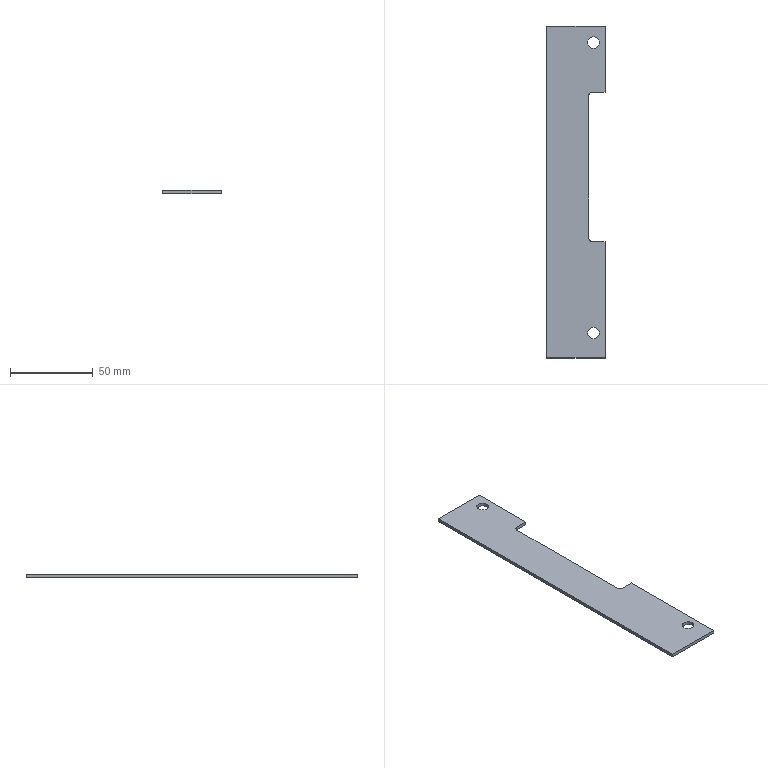Part | STEP file | 1_id642_x_t | 1 solid | 16 faces | box 35 x 200 x 2 mm | volume 12091 mm3 | plane 10 | cylinder 6 | commonest cylinder face diameters 7 x4 4 x2
STEP:
#1=CARTESIAN_POINT('',(0.,0.,0.));
#2=DIRECTION('',(0.,0.,1.));
#3=DIRECTION('',(1.,0.,0.));
#4=AXIS2_PLACEMENT_3D('',#1,#2,#3);
#5=CARTESIAN_POINT('',(533.775,132.525,-88.));
#6=VERTEX_POINT('',#5);
#7=CARTESIAN_POINT('',(531.775,134.525,-88.));
#8=VERTEX_POINT('',#7);
#9=CARTESIAN_POINT('',(533.775,134.525,-88.));
#10=DIRECTION('',(0.,0.,-1.));
#11=DIRECTION('',(0.,-1.,0.));
#12=AXIS2_PLACEMENT_3D('',#9,#10,#11);
#13=CIRCLE('',#12,2.);
#14=CARTESIAN_POINT('',(541.55,307.352,-88.));
#15=DIRECTION('',(0.,0.,1.));
#16=DIRECTION('',(1.,0.,0.));
#17=AXIS2_PLACEMENT_3D('',#14,#15,#16);
#18=PLANE('',#17);
#19=CARTESIAN_POINT('',(-7.775,-174.827));
#20=CARTESIAN_POINT('',(-11.239,-174.827));
#21=CARTESIAN_POINT('',(-9.507,-171.827));
#22=CARTESIAN_POINT('',(-7.775,-168.827));
#23=CARTESIAN_POINT('',(-6.043,-171.827));
#24=CARTESIAN_POINT('',(-4.311,-174.827));
#25=CARTESIAN_POINT('',(-7.775,-174.827));
#26=(BOUNDED_CURVE()B_SPLINE_CURVE(2,(#19,#20,#21,#22,#23,#24,#25),.UNSPECIFIED.,.T.,.F.)B_SPLINE_CURVE_WITH_KNOTS((1,2,2,2,2,1),(-2.094,0.,2.094,4.189,6.283,8.378),.UNSPECIFIED.)CURVE()GEOMETRIC_REPRESENTATION_ITEM()RATIONAL_B_SPLINE_CURVE((1.,0.5,1.,0.5,1.,0.5,1.))REPRESENTATION_ITEM(''));
#27=(GEOMETRIC_REPRESENTATION_CONTEXT(2)PARAMETRIC_REPRESENTATION_CONTEXT()REPRESENTATION_CONTEXT('',''));
#28=DEFINITIONAL_REPRESENTATION('',(#26),#27);
#29=PCURVE('',#18,#28);
#30=CARTESIAN_POINT('',(533.775,134.525,-92.));
#31=DIRECTION('',(0.,0.,-1.));
#32=DIRECTION('',(1.,0.,0.));
#33=AXIS2_PLACEMENT_3D('',#30,#31,#32);
#34=CYLINDRICAL_SURFACE('',#33,2.);
#35=CARTESIAN_POINT('',(1.571,-4.));
#36=DIRECTION('',(1.,0.));
#37=VECTOR('',#36,1.);
#38=LINE('',#35,#37);
#39=(GEOMETRIC_REPRESENTATION_CONTEXT(2)PARAMETRIC_REPRESENTATION_CONTEXT()REPRESENTATION_CONTEXT('',''));
#40=DEFINITIONAL_REPRESENTATION('',(#38),#39);
#41=PCURVE('',#34,#40);
#42=SURFACE_CURVE('',#13,(#29,#41),.PCURVE_S1.);
#43=EDGE_CURVE('',#6,#8,#42,.T.);
#44=ORIENTED_EDGE('',*,*,#43,.T.);
#45=CARTESIAN_POINT('',(531.775,220.475,-88.));
#46=VERTEX_POINT('',#45);
#47=CARTESIAN_POINT('',(531.775,134.525,-88.));
#48=DIRECTION('',(0.,1.,0.));
#49=VECTOR('',#48,1.);
#50=LINE('',#47,#49);
#51=CARTESIAN_POINT('',(-9.775,-172.827));
#52=DIRECTION('',(0.,1.));
#53=VECTOR('',#52,1.);
#54=LINE('',#51,#53);
#55=(GEOMETRIC_REPRESENTATION_CONTEXT(2)PARAMETRIC_REPRESENTATION_CONTEXT()REPRESENTATION_CONTEXT('',''));
#56=DEFINITIONAL_REPRESENTATION('',(#54),#55);
#57=PCURVE('',#18,#56);
#58=CARTESIAN_POINT('',(531.775,177.5,-92.));
#59=DIRECTION('',(-1.,0.,0.));
#60=DIRECTION('',(0.,0.,-1.));
#61=AXIS2_PLACEMENT_3D('',#58,#59,#60);
#62=PLANE('',#61);
#63=CARTESIAN_POINT('',(-4.,42.975));
#64=DIRECTION('',(0.,-1.));
#65=VECTOR('',#64,1.);
#66=LINE('',#63,#65);
#67=(GEOMETRIC_REPRESENTATION_CONTEXT(2)PARAMETRIC_REPRESENTATION_CONTEXT()REPRESENTATION_CONTEXT('',''));
#68=DEFINITIONAL_REPRESENTATION('',(#66),#67);
#69=PCURVE('',#62,#68);
#70=SURFACE_CURVE('',#50,(#57,#69),.PCURVE_S1.);
#71=EDGE_CURVE('',#8,#46,#70,.T.);
#72=ORIENTED_EDGE('',*,*,#71,.T.);
#73=CARTESIAN_POINT('',(533.775,222.475,-88.));
#74=VERTEX_POINT('',#73);
#75=CARTESIAN_POINT('',(533.775,220.475,-88.));
#76=DIRECTION('',(0.,0.,-1.));
#77=DIRECTION('',(-1.,0.,0.));
#78=AXIS2_PLACEMENT_3D('',#75,#76,#77);
#79=CIRCLE('',#78,2.);
#80=CARTESIAN_POINT('',(-9.775,-86.877));
#81=CARTESIAN_POINT('',(-9.775,-83.413));
#82=CARTESIAN_POINT('',(-6.775,-85.145));
#83=CARTESIAN_POINT('',(-3.775,-86.877));
#84=CARTESIAN_POINT('',(-6.775,-88.609));
#85=CARTESIAN_POINT('',(-9.775,-90.341));
#86=CARTESIAN_POINT('',(-9.775,-86.877));
#87=(BOUNDED_CURVE()B_SPLINE_CURVE(2,(#80,#81,#82,#83,#84,#85,#86),.UNSPECIFIED.,.T.,.F.)B_SPLINE_CURVE_WITH_KNOTS((1,2,2,2,2,1),(-2.094,0.,2.094,4.189,6.283,8.378),.UNSPECIFIED.)CURVE()GEOMETRIC_REPRESENTATION_ITEM()RATIONAL_B_SPLINE_CURVE((1.,0.5,1.,0.5,1.,0.5,1.))REPRESENTATION_ITEM(''));
#88=(GEOMETRIC_REPRESENTATION_CONTEXT(2)PARAMETRIC_REPRESENTATION_CONTEXT()REPRESENTATION_CONTEXT('',''));
#89=DEFINITIONAL_REPRESENTATION('',(#87),#88);
#90=PCURVE('',#18,#89);
#91=CARTESIAN_POINT('',(533.775,220.475,-92.));
#92=DIRECTION('',(0.,0.,-1.));
#93=DIRECTION('',(1.,0.,0.));
#94=AXIS2_PLACEMENT_3D('',#91,#92,#93);
#95=CYLINDRICAL_SURFACE('',#94,2.);
#96=CARTESIAN_POINT('',(3.142,-4.));
#97=DIRECTION('',(1.,0.));
#98=VECTOR('',#97,1.);
#99=LINE('',#96,#98);
#100=(GEOMETRIC_REPRESENTATION_CONTEXT(2)PARAMETRIC_REPRESENTATION_CONTEXT()REPRESENTATION_CONTEXT('',''));
#101=DEFINITIONAL_REPRESENTATION('',(#99),#100);
#102=PCURVE('',#95,#101);
#103=SURFACE_CURVE('',#79,(#90,#102),.PCURVE_S1.);
#104=EDGE_CURVE('',#46,#74,#103,.T.);
#105=ORIENTED_EDGE('',*,*,#104,.T.);
#106=CARTESIAN_POINT('',(541.55,222.475,-88.));
#107=VERTEX_POINT('',#106);
#108=CARTESIAN_POINT('',(533.775,222.475,-88.));
#109=DIRECTION('',(1.,0.,0.));
#110=VECTOR('',#109,1.);
#111=LINE('',#108,#110);
#112=CARTESIAN_POINT('',(-7.775,-84.877));
#113=DIRECTION('',(1.,0.));
#114=VECTOR('',#113,1.);
#115=LINE('',#112,#114);
#116=(GEOMETRIC_REPRESENTATION_CONTEXT(2)PARAMETRIC_REPRESENTATION_CONTEXT()REPRESENTATION_CONTEXT('',''));
#117=DEFINITIONAL_REPRESENTATION('',(#115),#116);
#118=PCURVE('',#18,#117);
#119=CARTESIAN_POINT('',(537.663,222.475,-92.));
#120=DIRECTION('',(0.,1.,0.));
#121=DIRECTION('',(0.,0.,-1.));
#122=AXIS2_PLACEMENT_3D('',#119,#120,#121);
#123=PLANE('',#122);
#124=CARTESIAN_POINT('',(-4.,3.888));
#125=DIRECTION('',(0.,-1.));
#126=VECTOR('',#125,1.);
#127=LINE('',#124,#126);
#128=(GEOMETRIC_REPRESENTATION_CONTEXT(2)PARAMETRIC_REPRESENTATION_CONTEXT()REPRESENTATION_CONTEXT('',''));
#129=DEFINITIONAL_REPRESENTATION('',(#127),#128);
#130=PCURVE('',#123,#129);
#131=SURFACE_CURVE('',#111,(#118,#130),.PCURVE_S1.);
#132=EDGE_CURVE('',#74,#107,#131,.T.);
#133=ORIENTED_EDGE('',*,*,#132,.T.);
#134=CARTESIAN_POINT('',(541.55,262.352,-88.));
#135=VERTEX_POINT('',#134);
#136=CARTESIAN_POINT('',(541.55,262.352,-88.));
#137=DIRECTION('',(0.,-1.,0.));
#138=VECTOR('',#137,1.);
#139=LINE('',#136,#138);
#140=CARTESIAN_POINT('',(0.,-45.));
#141=DIRECTION('',(0.,-1.));
#142=VECTOR('',#141,1.);
#143=LINE('',#140,#142);
#144=(GEOMETRIC_REPRESENTATION_CONTEXT(2)PARAMETRIC_REPRESENTATION_CONTEXT()REPRESENTATION_CONTEXT('',''));
#145=DEFINITIONAL_REPRESENTATION('',(#143),#144);
#146=PCURVE('',#18,#145);
#147=CARTESIAN_POINT('',(541.55,62.352,-88.));
#148=DIRECTION('',(-1.,0.,0.));
#149=DIRECTION('',(0.,-1.,0.));
#150=AXIS2_PLACEMENT_3D('',#147,#148,#149);
#151=PLANE('',#150);
#152=CARTESIAN_POINT('',(-200.,0.));
#153=DIRECTION('',(1.,0.));
#154=VECTOR('',#153,1.);
#155=LINE('',#152,#154);
#156=(GEOMETRIC_REPRESENTATION_CONTEXT(2)PARAMETRIC_REPRESENTATION_CONTEXT()REPRESENTATION_CONTEXT('',''));
#157=DEFINITIONAL_REPRESENTATION('',(#155),#156);
#158=PCURVE('',#151,#157);
#159=SURFACE_CURVE('',#139,(#146,#158),.PCURVE_S1.);
#160=EDGE_CURVE('',#135,#107,#159,.T.);
#161=ORIENTED_EDGE('',*,*,#160,.F.);
#162=CARTESIAN_POINT('',(506.55,262.352,-88.));
#163=VERTEX_POINT('',#162);
#164=CARTESIAN_POINT('',(506.55,262.352,-88.));
#165=DIRECTION('',(1.,0.,0.));
#166=VECTOR('',#165,1.);
#167=LINE('',#164,#166);
#168=CARTESIAN_POINT('',(-35.,-45.));
#169=DIRECTION('',(1.,0.));
#170=VECTOR('',#169,1.);
#171=LINE('',#168,#170);
#172=(GEOMETRIC_REPRESENTATION_CONTEXT(2)PARAMETRIC_REPRESENTATION_CONTEXT()REPRESENTATION_CONTEXT('',''));
#173=DEFINITIONAL_REPRESENTATION('',(#171),#172);
#174=PCURVE('',#18,#173);
#175=CARTESIAN_POINT('',(541.55,262.352,-88.));
#176=DIRECTION('',(0.,-1.,0.));
#177=DIRECTION('',(0.,0.,1.));
#178=AXIS2_PLACEMENT_3D('',#175,#176,#177);
#179=PLANE('',#178);
#180=CARTESIAN_POINT('',(0.,35.));
#181=DIRECTION('',(0.,-1.));
#182=VECTOR('',#181,1.);
#183=LINE('',#180,#182);
#184=(GEOMETRIC_REPRESENTATION_CONTEXT(2)PARAMETRIC_REPRESENTATION_CONTEXT()REPRESENTATION_CONTEXT('',''));
#185=DEFINITIONAL_REPRESENTATION('',(#183),#184);
#186=PCURVE('',#179,#185);
#187=SURFACE_CURVE('',#167,(#174,#186),.PCURVE_S1.);
#188=EDGE_CURVE('',#163,#135,#187,.T.);
#189=ORIENTED_EDGE('',*,*,#188,.F.);
#190=CARTESIAN_POINT('',(506.55,62.352,-88.));
#191=VERTEX_POINT('',#190);
#192=CARTESIAN_POINT('',(506.55,62.352,-88.));
#193=DIRECTION('',(0.,1.,0.));
#194=VECTOR('',#193,1.);
#195=LINE('',#192,#194);
#196=CARTESIAN_POINT('',(-35.,-245.));
#197=DIRECTION('',(0.,1.));
#198=VECTOR('',#197,1.);
#199=LINE('',#196,#198);
#200=(GEOMETRIC_REPRESENTATION_CONTEXT(2)PARAMETRIC_REPRESENTATION_CONTEXT()REPRESENTATION_CONTEXT('',''));
#201=DEFINITIONAL_REPRESENTATION('',(#199),#200);
#202=PCURVE('',#18,#201);
#203=CARTESIAN_POINT('',(506.55,177.5,-52.5));
#204=DIRECTION('',(-1.,0.,0.));
#205=DIRECTION('',(0.,0.,-1.));
#206=AXIS2_PLACEMENT_3D('',#203,#204,#205);
#207=PLANE('',#206);
#208=CARTESIAN_POINT('',(35.5,115.148));
#209=DIRECTION('',(0.,-1.));
#210=VECTOR('',#209,1.);
#211=LINE('',#208,#210);
#212=(GEOMETRIC_REPRESENTATION_CONTEXT(2)PARAMETRIC_REPRESENTATION_CONTEXT()REPRESENTATION_CONTEXT('',''));
#213=DEFINITIONAL_REPRESENTATION('',(#211),#212);
#214=PCURVE('',#207,#213);
#215=SURFACE_CURVE('',#195,(#202,#214),.PCURVE_S1.);
#216=EDGE_CURVE('',#191,#163,#215,.T.);
#217=ORIENTED_EDGE('',*,*,#216,.F.);
#218=CARTESIAN_POINT('',(541.55,62.352,-88.));
#219=VERTEX_POINT('',#218);
#220=CARTESIAN_POINT('',(541.55,62.352,-88.));
#221=DIRECTION('',(-1.,0.,0.));
#222=VECTOR('',#221,1.);
#223=LINE('',#220,#222);
#224=CARTESIAN_POINT('',(0.,-245.));
#225=DIRECTION('',(-1.,0.));
#226=VECTOR('',#225,1.);
#227=LINE('',#224,#226);
#228=(GEOMETRIC_REPRESENTATION_CONTEXT(2)PARAMETRIC_REPRESENTATION_CONTEXT()REPRESENTATION_CONTEXT('',''));
#229=DEFINITIONAL_REPRESENTATION('',(#227),#228);
#230=PCURVE('',#18,#229);
#231=CARTESIAN_POINT('',(496.55,62.352,-88.));
#232=DIRECTION('',(0.,1.,0.));
#233=DIRECTION('',(0.,0.,-1.));
#234=AXIS2_PLACEMENT_3D('',#231,#232,#233);
#235=PLANE('',#234);
#236=CARTESIAN_POINT('',(0.,-45.));
#237=DIRECTION('',(0.,1.));
#238=VECTOR('',#237,1.);
#239=LINE('',#236,#238);
#240=(GEOMETRIC_REPRESENTATION_CONTEXT(2)PARAMETRIC_REPRESENTATION_CONTEXT()REPRESENTATION_CONTEXT('',''));
#241=DEFINITIONAL_REPRESENTATION('',(#239),#240);
#242=PCURVE('',#235,#241);
#243=SURFACE_CURVE('',#223,(#230,#242),.PCURVE_S1.);
#244=EDGE_CURVE('',#219,#191,#243,.T.);
#245=ORIENTED_EDGE('',*,*,#244,.F.);
#246=CARTESIAN_POINT('',(541.55,132.525,-88.));
#247=VERTEX_POINT('',#246);
#248=CARTESIAN_POINT('',(541.55,132.525,-88.));
#249=DIRECTION('',(0.,-1.,0.));
#250=VECTOR('',#249,1.);
#251=LINE('',#248,#250);
#252=CARTESIAN_POINT('',(0.,-174.827));
#253=DIRECTION('',(0.,-1.));
#254=VECTOR('',#253,1.);
#255=LINE('',#252,#254);
#256=(GEOMETRIC_REPRESENTATION_CONTEXT(2)PARAMETRIC_REPRESENTATION_CONTEXT()REPRESENTATION_CONTEXT('',''));
#257=DEFINITIONAL_REPRESENTATION('',(#255),#256);
#258=PCURVE('',#18,#257);
#259=CARTESIAN_POINT('',(541.55,62.352,-88.));
#260=DIRECTION('',(-1.,0.,0.));
#261=DIRECTION('',(0.,-1.,0.));
#262=AXIS2_PLACEMENT_3D('',#259,#260,#261);
#263=PLANE('',#262);
#264=CARTESIAN_POINT('',(-70.173,0.));
#265=DIRECTION('',(1.,0.));
#266=VECTOR('',#265,1.);
#267=LINE('',#264,#266);
#268=(GEOMETRIC_REPRESENTATION_CONTEXT(2)PARAMETRIC_REPRESENTATION_CONTEXT()REPRESENTATION_CONTEXT('',''));
#269=DEFINITIONAL_REPRESENTATION('',(#267),#268);
#270=PCURVE('',#263,#269);
#271=SURFACE_CURVE('',#251,(#258,#270),.PCURVE_S1.);
#272=EDGE_CURVE('',#247,#219,#271,.T.);
#273=ORIENTED_EDGE('',*,*,#272,.F.);
#274=CARTESIAN_POINT('',(541.55,132.525,-88.));
#275=DIRECTION('',(-1.,0.,0.));
#276=VECTOR('',#275,1.);
#277=LINE('',#274,#276);
#278=CARTESIAN_POINT('',(0.,-174.827));
#279=DIRECTION('',(-1.,0.));
#280=VECTOR('',#279,1.);
#281=LINE('',#278,#280);
#282=(GEOMETRIC_REPRESENTATION_CONTEXT(2)PARAMETRIC_REPRESENTATION_CONTEXT()REPRESENTATION_CONTEXT('',''));
#283=DEFINITIONAL_REPRESENTATION('',(#281),#282);
#284=PCURVE('',#18,#283);
#285=CARTESIAN_POINT('',(537.663,132.525,-92.));
#286=DIRECTION('',(0.,-1.,0.));
#287=DIRECTION('',(0.,0.,1.));
#288=AXIS2_PLACEMENT_3D('',#285,#286,#287);
#289=PLANE('',#288);
#290=CARTESIAN_POINT('',(4.,-3.888));
#291=DIRECTION('',(0.,1.));
#292=VECTOR('',#291,1.);
#293=LINE('',#290,#292);
#294=(GEOMETRIC_REPRESENTATION_CONTEXT(2)PARAMETRIC_REPRESENTATION_CONTEXT()REPRESENTATION_CONTEXT('',''));
#295=DEFINITIONAL_REPRESENTATION('',(#293),#294);
#296=PCURVE('',#289,#295);
#297=SURFACE_CURVE('',#277,(#284,#296),.PCURVE_S1.);
#298=EDGE_CURVE('',#247,#6,#297,.T.);
#299=ORIENTED_EDGE('',*,*,#298,.T.);
#300=EDGE_LOOP('',(#44,#72,#105,#133,#161,#189,#217,#245,#273,#299));
#301=FACE_BOUND('',#300,.T.);
#302=CARTESIAN_POINT('',(531.05,77.352,-88.));
#303=VERTEX_POINT('',#302);
#304=CARTESIAN_POINT('',(538.05,77.352,-88.));
#305=VERTEX_POINT('',#304);
#306=CARTESIAN_POINT('',(534.55,77.352,-88.));
#307=DIRECTION('',(0.,0.,-1.));
#308=DIRECTION('',(-1.,0.,0.));
#309=AXIS2_PLACEMENT_3D('',#306,#307,#308);
#310=CIRCLE('',#309,3.5);
#311=CARTESIAN_POINT('',(-10.5,-230.));
#312=CARTESIAN_POINT('',(-10.5,-223.938));
#313=CARTESIAN_POINT('',(-5.25,-226.969));
#314=CARTESIAN_POINT('',(0.,-230.));
#315=CARTESIAN_POINT('',(-5.25,-233.031));
#316=CARTESIAN_POINT('',(-10.5,-236.062));
#317=CARTESIAN_POINT('',(-10.5,-230.));
#318=(BOUNDED_CURVE()B_SPLINE_CURVE(2,(#311,#312,#313,#314,#315,#316,#317),.UNSPECIFIED.,.T.,.F.)B_SPLINE_CURVE_WITH_KNOTS((1,2,2,2,2,1),(-2.094,0.,2.094,4.189,6.283,8.378),.UNSPECIFIED.)CURVE()GEOMETRIC_REPRESENTATION_ITEM()RATIONAL_B_SPLINE_CURVE((1.,0.5,1.,0.5,1.,0.5,1.))REPRESENTATION_ITEM(''));
#319=(GEOMETRIC_REPRESENTATION_CONTEXT(2)PARAMETRIC_REPRESENTATION_CONTEXT()REPRESENTATION_CONTEXT('',''));
#320=DEFINITIONAL_REPRESENTATION('',(#318),#319);
#321=PCURVE('',#18,#320);
#322=CARTESIAN_POINT('',(534.55,77.352,-88.));
#323=DIRECTION('',(0.,0.,-1.));
#324=DIRECTION('',(-1.,0.,0.));
#325=AXIS2_PLACEMENT_3D('',#322,#323,#324);
#326=CYLINDRICAL_SURFACE('',#325,3.5);
#327=CARTESIAN_POINT('',(0.,0.));
#328=DIRECTION('',(1.,0.));
#329=VECTOR('',#328,1.);
#330=LINE('',#327,#329);
#331=(GEOMETRIC_REPRESENTATION_CONTEXT(2)PARAMETRIC_REPRESENTATION_CONTEXT()REPRESENTATION_CONTEXT('',''));
#332=DEFINITIONAL_REPRESENTATION('',(#330),#331);
#333=PCURVE('',#326,#332);
#334=SURFACE_CURVE('',#310,(#321,#333),.PCURVE_S1.);
#335=EDGE_CURVE('',#303,#305,#334,.T.);
#336=ORIENTED_EDGE('',*,*,#335,.T.);
#337=CARTESIAN_POINT('',(534.55,77.352,-88.));
#338=DIRECTION('',(0.,0.,-1.));
#339=DIRECTION('',(1.,0.,0.));
#340=AXIS2_PLACEMENT_3D('',#337,#338,#339);
#341=CIRCLE('',#340,3.5);
#342=CARTESIAN_POINT('',(-3.5,-230.));
#343=CARTESIAN_POINT('',(-3.5,-236.062));
#344=CARTESIAN_POINT('',(-8.75,-233.031));
#345=CARTESIAN_POINT('',(-14.,-230.));
#346=CARTESIAN_POINT('',(-8.75,-226.969));
#347=CARTESIAN_POINT('',(-3.5,-223.938));
#348=CARTESIAN_POINT('',(-3.5,-230.));
#349=(BOUNDED_CURVE()B_SPLINE_CURVE(2,(#342,#343,#344,#345,#346,#347,#348),.UNSPECIFIED.,.T.,.F.)B_SPLINE_CURVE_WITH_KNOTS((1,2,2,2,2,1),(-2.094,0.,2.094,4.189,6.283,8.378),.UNSPECIFIED.)CURVE()GEOMETRIC_REPRESENTATION_ITEM()RATIONAL_B_SPLINE_CURVE((1.,0.5,1.,0.5,1.,0.5,1.))REPRESENTATION_ITEM(''));
#350=(GEOMETRIC_REPRESENTATION_CONTEXT(2)PARAMETRIC_REPRESENTATION_CONTEXT()REPRESENTATION_CONTEXT('',''));
#351=DEFINITIONAL_REPRESENTATION('',(#349),#350);
#352=PCURVE('',#18,#351);
#353=CARTESIAN_POINT('',(534.55,77.352,-88.));
#354=DIRECTION('',(0.,0.,-1.));
#355=DIRECTION('',(-1.,0.,0.));
#356=AXIS2_PLACEMENT_3D('',#353,#354,#355);
#357=CYLINDRICAL_SURFACE('',#356,3.5);
#358=CARTESIAN_POINT('',(3.142,0.));
#359=DIRECTION('',(1.,0.));
#360=VECTOR('',#359,1.);
#361=LINE('',#358,#360);
#362=(GEOMETRIC_REPRESENTATION_CONTEXT(2)PARAMETRIC_REPRESENTATION_CONTEXT()REPRESENTATION_CONTEXT('',''));
#363=DEFINITIONAL_REPRESENTATION('',(#361),#362);
#364=PCURVE('',#357,#363);
#365=SURFACE_CURVE('',#341,(#352,#364),.PCURVE_S1.);
#366=EDGE_CURVE('',#305,#303,#365,.T.);
#367=ORIENTED_EDGE('',*,*,#366,.T.);
#368=EDGE_LOOP('',(#336,#367));
#369=FACE_BOUND('',#368,.T.);
#370=CARTESIAN_POINT('',(531.05,252.352,-88.));
#371=VERTEX_POINT('',#370);
#372=CARTESIAN_POINT('',(538.05,252.352,-88.));
#373=VERTEX_POINT('',#372);
#374=CARTESIAN_POINT('',(534.55,252.352,-88.));
#375=DIRECTION('',(0.,0.,-1.));
#376=DIRECTION('',(-1.,0.,0.));
#377=AXIS2_PLACEMENT_3D('',#374,#375,#376);
#378=CIRCLE('',#377,3.5);
#379=CARTESIAN_POINT('',(-10.5,-55.));
#380=CARTESIAN_POINT('',(-10.5,-48.938));
#381=CARTESIAN_POINT('',(-5.25,-51.969));
#382=CARTESIAN_POINT('',(0.,-55.));
#383=CARTESIAN_POINT('',(-5.25,-58.031));
#384=CARTESIAN_POINT('',(-10.5,-61.062));
#385=CARTESIAN_POINT('',(-10.5,-55.));
#386=(BOUNDED_CURVE()B_SPLINE_CURVE(2,(#379,#380,#381,#382,#383,#384,#385),.UNSPECIFIED.,.T.,.F.)B_SPLINE_CURVE_WITH_KNOTS((1,2,2,2,2,1),(-2.094,0.,2.094,4.189,6.283,8.378),.UNSPECIFIED.)CURVE()GEOMETRIC_REPRESENTATION_ITEM()RATIONAL_B_SPLINE_CURVE((1.,0.5,1.,0.5,1.,0.5,1.))REPRESENTATION_ITEM(''));
#387=(GEOMETRIC_REPRESENTATION_CONTEXT(2)PARAMETRIC_REPRESENTATION_CONTEXT()REPRESENTATION_CONTEXT('',''));
#388=DEFINITIONAL_REPRESENTATION('',(#386),#387);
#389=PCURVE('',#18,#388);
#390=CARTESIAN_POINT('',(534.55,252.352,-88.));
#391=DIRECTION('',(0.,0.,-1.));
#392=DIRECTION('',(-1.,0.,0.));
#393=AXIS2_PLACEMENT_3D('',#390,#391,#392);
#394=CYLINDRICAL_SURFACE('',#393,3.5);
#395=CARTESIAN_POINT('',(0.,0.));
#396=DIRECTION('',(1.,0.));
#397=VECTOR('',#396,1.);
#398=LINE('',#395,#397);
#399=(GEOMETRIC_REPRESENTATION_CONTEXT(2)PARAMETRIC_REPRESENTATION_CONTEXT()REPRESENTATION_CONTEXT('',''));
#400=DEFINITIONAL_REPRESENTATION('',(#398),#399);
#401=PCURVE('',#394,#400);
#402=SURFACE_CURVE('',#378,(#389,#401),.PCURVE_S1.);
#403=EDGE_CURVE('',#371,#373,#402,.T.);
#404=ORIENTED_EDGE('',*,*,#403,.T.);
#405=CARTESIAN_POINT('',(534.55,252.352,-88.));
#406=DIRECTION('',(0.,0.,-1.));
#407=DIRECTION('',(1.,0.,0.));
#408=AXIS2_PLACEMENT_3D('',#405,#406,#407);
#409=CIRCLE('',#408,3.5);
#410=CARTESIAN_POINT('',(-3.5,-55.));
#411=CARTESIAN_POINT('',(-3.5,-61.062));
#412=CARTESIAN_POINT('',(-8.75,-58.031));
#413=CARTESIAN_POINT('',(-14.,-55.));
#414=CARTESIAN_POINT('',(-8.75,-51.969));
#415=CARTESIAN_POINT('',(-3.5,-48.938));
#416=CARTESIAN_POINT('',(-3.5,-55.));
#417=(BOUNDED_CURVE()B_SPLINE_CURVE(2,(#410,#411,#412,#413,#414,#415,#416),.UNSPECIFIED.,.T.,.F.)B_SPLINE_CURVE_WITH_KNOTS((1,2,2,2,2,1),(-2.094,0.,2.094,4.189,6.283,8.378),.UNSPECIFIED.)CURVE()GEOMETRIC_REPRESENTATION_ITEM()RATIONAL_B_SPLINE_CURVE((1.,0.5,1.,0.5,1.,0.5,1.))REPRESENTATION_ITEM(''));
#418=(GEOMETRIC_REPRESENTATION_CONTEXT(2)PARAMETRIC_REPRESENTATION_CONTEXT()REPRESENTATION_CONTEXT('',''));
#419=DEFINITIONAL_REPRESENTATION('',(#417),#418);
#420=PCURVE('',#18,#419);
#421=CARTESIAN_POINT('',(534.55,252.352,-88.));
#422=DIRECTION('',(0.,0.,-1.));
#423=DIRECTION('',(-1.,0.,0.));
#424=AXIS2_PLACEMENT_3D('',#421,#422,#423);
#425=CYLINDRICAL_SURFACE('',#424,3.5);
#426=CARTESIAN_POINT('',(3.142,0.));
#427=DIRECTION('',(1.,0.));
#428=VECTOR('',#427,1.);
#429=LINE('',#426,#428);
#430=(GEOMETRIC_REPRESENTATION_CONTEXT(2)PARAMETRIC_REPRESENTATION_CONTEXT()REPRESENTATION_CONTEXT('',''));
#431=DEFINITIONAL_REPRESENTATION('',(#429),#430);
#432=PCURVE('',#425,#431);
#433=SURFACE_CURVE('',#409,(#420,#432),.PCURVE_S1.);
#434=EDGE_CURVE('',#373,#371,#433,.T.);
#435=ORIENTED_EDGE('',*,*,#434,.T.);
#436=EDGE_LOOP('',(#404,#435));
#437=FACE_BOUND('',#436,.T.);
#438=ADVANCED_FACE('',(#301,#369,#437),#18,.T.);
#439=CARTESIAN_POINT('',(533.775,132.525,-90.));
#440=VERTEX_POINT('',#439);
#441=CARTESIAN_POINT('',(533.775,132.525,-88.));
#442=DIRECTION('',(0.,0.,-1.));
#443=VECTOR('',#442,1.);
#444=LINE('',#441,#443);
#445=CARTESIAN_POINT('',(4.,3.888));
#446=DIRECTION('',(-1.,0.));
#447=VECTOR('',#446,1.);
#448=LINE('',#445,#447);
#449=(GEOMETRIC_REPRESENTATION_CONTEXT(2)PARAMETRIC_REPRESENTATION_CONTEXT()REPRESENTATION_CONTEXT('',''));
#450=DEFINITIONAL_REPRESENTATION('',(#448),#449);
#451=PCURVE('',#289,#450);
#452=CARTESIAN_POINT('',(1.571,-4.));
#453=DIRECTION('',(0.,1.));
#454=VECTOR('',#453,1.);
#455=LINE('',#452,#454);
#456=(GEOMETRIC_REPRESENTATION_CONTEXT(2)PARAMETRIC_REPRESENTATION_CONTEXT()REPRESENTATION_CONTEXT('',''));
#457=DEFINITIONAL_REPRESENTATION('',(#455),#456);
#458=PCURVE('',#34,#457);
#459=SURFACE_CURVE('',#444,(#451,#458),.PCURVE_S1.);
#460=EDGE_CURVE('',#6,#440,#459,.T.);
#461=ORIENTED_EDGE('',*,*,#460,.F.);
#462=ORIENTED_EDGE('',*,*,#298,.F.);
#463=CARTESIAN_POINT('',(541.55,132.525,-90.));
#464=VERTEX_POINT('',#463);
#465=CARTESIAN_POINT('',(541.55,132.525,-88.));
#466=DIRECTION('',(0.,0.,-1.));
#467=VECTOR('',#466,1.);
#468=LINE('',#465,#467);
#469=CARTESIAN_POINT('',(4.,-3.888));
#470=DIRECTION('',(-1.,0.));
#471=VECTOR('',#470,1.);
#472=LINE('',#469,#471);
#473=(GEOMETRIC_REPRESENTATION_CONTEXT(2)PARAMETRIC_REPRESENTATION_CONTEXT()REPRESENTATION_CONTEXT('',''));
#474=DEFINITIONAL_REPRESENTATION('',(#472),#473);
#475=PCURVE('',#289,#474);
#476=CARTESIAN_POINT('',(-70.173,0.));
#477=DIRECTION('',(0.,-1.));
#478=VECTOR('',#477,1.);
#479=LINE('',#476,#478);
#480=(GEOMETRIC_REPRESENTATION_CONTEXT(2)PARAMETRIC_REPRESENTATION_CONTEXT()REPRESENTATION_CONTEXT('',''));
#481=DEFINITIONAL_REPRESENTATION('',(#479),#480);
#482=PCURVE('',#263,#481);
#483=SURFACE_CURVE('',#468,(#475,#482),.PCURVE_S1.);
#484=EDGE_CURVE('',#247,#464,#483,.T.);
#485=ORIENTED_EDGE('',*,*,#484,.T.);
#486=CARTESIAN_POINT('',(541.55,132.525,-90.));
#487=DIRECTION('',(-1.,0.,0.));
#488=VECTOR('',#487,1.);
#489=LINE('',#486,#488);
#490=CARTESIAN_POINT('',(2.,-3.888));
#491=DIRECTION('',(0.,1.));
#492=VECTOR('',#491,1.);
#493=LINE('',#490,#492);
#494=(GEOMETRIC_REPRESENTATION_CONTEXT(2)PARAMETRIC_REPRESENTATION_CONTEXT()REPRESENTATION_CONTEXT('',''));
#495=DEFINITIONAL_REPRESENTATION('',(#493),#494);
#496=PCURVE('',#289,#495);
#497=CARTESIAN_POINT('',(541.55,307.352,-90.));
#498=DIRECTION('',(0.,0.,1.));
#499=DIRECTION('',(1.,0.,0.));
#500=AXIS2_PLACEMENT_3D('',#497,#498,#499);
#501=PLANE('',#500);
#502=CARTESIAN_POINT('',(0.,-174.827));
#503=DIRECTION('',(-1.,0.));
#504=VECTOR('',#503,1.);
#505=LINE('',#502,#504);
#506=(GEOMETRIC_REPRESENTATION_CONTEXT(2)PARAMETRIC_REPRESENTATION_CONTEXT()REPRESENTATION_CONTEXT('',''));
#507=DEFINITIONAL_REPRESENTATION('',(#505),#506);
#508=PCURVE('',#501,#507);
#509=SURFACE_CURVE('',#489,(#496,#508),.PCURVE_S1.);
#510=EDGE_CURVE('',#464,#440,#509,.T.);
#511=ORIENTED_EDGE('',*,*,#510,.T.);
#512=EDGE_LOOP('',(#461,#462,#485,#511));
#513=FACE_BOUND('',#512,.T.);
#514=ADVANCED_FACE('',(#513),#289,.F.);
#515=CARTESIAN_POINT('',(533.775,222.475,-90.));
#516=VERTEX_POINT('',#515);
#517=CARTESIAN_POINT('',(531.775,220.475,-90.));
#518=VERTEX_POINT('',#517);
#519=CARTESIAN_POINT('',(533.775,220.475,-90.));
#520=DIRECTION('',(0.,0.,1.));
#521=DIRECTION('',(0.,1.,0.));
#522=AXIS2_PLACEMENT_3D('',#519,#520,#521);
#523=CIRCLE('',#522,2.);
#524=CARTESIAN_POINT('',(-7.775,-86.877));
#525=DIRECTION('',(0.,1.));
#526=AXIS2_PLACEMENT_2D('',#524,#525);
#527=CIRCLE('',#526,2.);
#528=(GEOMETRIC_REPRESENTATION_CONTEXT(2)PARAMETRIC_REPRESENTATION_CONTEXT()REPRESENTATION_CONTEXT('',''));
#529=DEFINITIONAL_REPRESENTATION('',(#527),#528);
#530=PCURVE('',#501,#529);
#531=CARTESIAN_POINT('',(4.712,-2.));
#532=DIRECTION('',(-1.,0.));
#533=VECTOR('',#532,1.);
#534=LINE('',#531,#533);
#535=(GEOMETRIC_REPRESENTATION_CONTEXT(2)PARAMETRIC_REPRESENTATION_CONTEXT()REPRESENTATION_CONTEXT('',''));
#536=DEFINITIONAL_REPRESENTATION('',(#534),#535);
#537=PCURVE('',#95,#536);
#538=SURFACE_CURVE('',#523,(#530,#537),.PCURVE_S1.);
#539=EDGE_CURVE('',#516,#518,#538,.T.);
#540=ORIENTED_EDGE('',*,*,#539,.T.);
#541=CARTESIAN_POINT('',(531.775,134.525,-90.));
#542=VERTEX_POINT('',#541);
#543=CARTESIAN_POINT('',(531.775,134.525,-90.));
#544=DIRECTION('',(0.,1.,0.));
#545=VECTOR('',#544,1.);
#546=LINE('',#543,#545);
#547=CARTESIAN_POINT('',(-9.775,-172.827));
#548=DIRECTION('',(0.,1.));
#549=VECTOR('',#548,1.);
#550=LINE('',#547,#549);
#551=(GEOMETRIC_REPRESENTATION_CONTEXT(2)PARAMETRIC_REPRESENTATION_CONTEXT()REPRESENTATION_CONTEXT('',''));
#552=DEFINITIONAL_REPRESENTATION('',(#550),#551);
#553=PCURVE('',#501,#552);
#554=CARTESIAN_POINT('',(-2.,42.975));
#555=DIRECTION('',(0.,-1.));
#556=VECTOR('',#555,1.);
#557=LINE('',#554,#556);
#558=(GEOMETRIC_REPRESENTATION_CONTEXT(2)PARAMETRIC_REPRESENTATION_CONTEXT()REPRESENTATION_CONTEXT('',''));
#559=DEFINITIONAL_REPRESENTATION('',(#557),#558);
#560=PCURVE('',#62,#559);
#561=SURFACE_CURVE('',#546,(#553,#560),.PCURVE_S1.);
#562=EDGE_CURVE('',#542,#518,#561,.T.);
#563=ORIENTED_EDGE('',*,*,#562,.F.);
#564=CARTESIAN_POINT('',(533.775,134.525,-90.));
#565=DIRECTION('',(0.,0.,1.));
#566=DIRECTION('',(-1.,0.,0.));
#567=AXIS2_PLACEMENT_3D('',#564,#565,#566);
#568=CIRCLE('',#567,2.);
#569=CARTESIAN_POINT('',(-7.775,-172.827));
#570=DIRECTION('',(-1.,0.));
#571=AXIS2_PLACEMENT_2D('',#569,#570);
#572=CIRCLE('',#571,2.);
#573=(GEOMETRIC_REPRESENTATION_CONTEXT(2)PARAMETRIC_REPRESENTATION_CONTEXT()REPRESENTATION_CONTEXT('',''));
#574=DEFINITIONAL_REPRESENTATION('',(#572),#573);
#575=PCURVE('',#501,#574);
#576=CARTESIAN_POINT('',(3.142,-2.));
#577=DIRECTION('',(-1.,0.));
#578=VECTOR('',#577,1.);
#579=LINE('',#576,#578);
#580=(GEOMETRIC_REPRESENTATION_CONTEXT(2)PARAMETRIC_REPRESENTATION_CONTEXT()REPRESENTATION_CONTEXT('',''));
#581=DEFINITIONAL_REPRESENTATION('',(#579),#580);
#582=PCURVE('',#34,#581);
#583=SURFACE_CURVE('',#568,(#575,#582),.PCURVE_S1.);
#584=EDGE_CURVE('',#542,#440,#583,.T.);
#585=ORIENTED_EDGE('',*,*,#584,.T.);
#586=ORIENTED_EDGE('',*,*,#510,.F.);
#587=CARTESIAN_POINT('',(541.55,62.352,-90.));
#588=VERTEX_POINT('',#587);
#589=CARTESIAN_POINT('',(541.55,132.525,-90.));
#590=DIRECTION('',(0.,-1.,0.));
#591=VECTOR('',#590,1.);
#592=LINE('',#589,#591);
#593=CARTESIAN_POINT('',(0.,-174.827));
#594=DIRECTION('',(0.,-1.));
#595=VECTOR('',#594,1.);
#596=LINE('',#593,#595);
#597=(GEOMETRIC_REPRESENTATION_CONTEXT(2)PARAMETRIC_REPRESENTATION_CONTEXT()REPRESENTATION_CONTEXT('',''));
#598=DEFINITIONAL_REPRESENTATION('',(#596),#597);
#599=PCURVE('',#501,#598);
#600=CARTESIAN_POINT('',(-70.173,-2.));
#601=DIRECTION('',(1.,0.));
#602=VECTOR('',#601,1.);
#603=LINE('',#600,#602);
#604=(GEOMETRIC_REPRESENTATION_CONTEXT(2)PARAMETRIC_REPRESENTATION_CONTEXT()REPRESENTATION_CONTEXT('',''));
#605=DEFINITIONAL_REPRESENTATION('',(#603),#604);
#606=PCURVE('',#263,#605);
#607=SURFACE_CURVE('',#592,(#599,#606),.PCURVE_S1.);
#608=EDGE_CURVE('',#464,#588,#607,.T.);
#609=ORIENTED_EDGE('',*,*,#608,.T.);
#610=CARTESIAN_POINT('',(506.55,62.352,-90.));
#611=VERTEX_POINT('',#610);
#612=CARTESIAN_POINT('',(541.55,62.352,-90.));
#613=DIRECTION('',(-1.,0.,0.));
#614=VECTOR('',#613,1.);
#615=LINE('',#612,#614);
#616=CARTESIAN_POINT('',(0.,-245.));
#617=DIRECTION('',(-1.,0.));
#618=VECTOR('',#617,1.);
#619=LINE('',#616,#618);
#620=(GEOMETRIC_REPRESENTATION_CONTEXT(2)PARAMETRIC_REPRESENTATION_CONTEXT()REPRESENTATION_CONTEXT('',''));
#621=DEFINITIONAL_REPRESENTATION('',(#619),#620);
#622=PCURVE('',#501,#621);
#623=CARTESIAN_POINT('',(2.,-45.));
#624=DIRECTION('',(0.,1.));
#625=VECTOR('',#624,1.);
#626=LINE('',#623,#625);
#627=(GEOMETRIC_REPRESENTATION_CONTEXT(2)PARAMETRIC_REPRESENTATION_CONTEXT()REPRESENTATION_CONTEXT('',''));
#628=DEFINITIONAL_REPRESENTATION('',(#626),#627);
#629=PCURVE('',#235,#628);
#630=SURFACE_CURVE('',#615,(#622,#629),.PCURVE_S1.);
#631=EDGE_CURVE('',#588,#611,#630,.T.);
#632=ORIENTED_EDGE('',*,*,#631,.T.);
#633=CARTESIAN_POINT('',(506.55,262.352,-90.));
#634=VERTEX_POINT('',#633);
#635=CARTESIAN_POINT('',(506.55,62.352,-90.));
#636=DIRECTION('',(0.,1.,0.));
#637=VECTOR('',#636,1.);
#638=LINE('',#635,#637);
#639=CARTESIAN_POINT('',(-35.,-245.));
#640=DIRECTION('',(0.,1.));
#641=VECTOR('',#640,1.);
#642=LINE('',#639,#641);
#643=(GEOMETRIC_REPRESENTATION_CONTEXT(2)PARAMETRIC_REPRESENTATION_CONTEXT()REPRESENTATION_CONTEXT('',''));
#644=DEFINITIONAL_REPRESENTATION('',(#642),#643);
#645=PCURVE('',#501,#644);
#646=CARTESIAN_POINT('',(37.5,115.148));
#647=DIRECTION('',(0.,-1.));
#648=VECTOR('',#647,1.);
#649=LINE('',#646,#648);
#650=(GEOMETRIC_REPRESENTATION_CONTEXT(2)PARAMETRIC_REPRESENTATION_CONTEXT()REPRESENTATION_CONTEXT('',''));
#651=DEFINITIONAL_REPRESENTATION('',(#649),#650);
#652=PCURVE('',#207,#651);
#653=SURFACE_CURVE('',#638,(#645,#652),.PCURVE_S1.);
#654=EDGE_CURVE('',#611,#634,#653,.T.);
#655=ORIENTED_EDGE('',*,*,#654,.T.);
#656=CARTESIAN_POINT('',(541.55,262.352,-90.));
#657=VERTEX_POINT('',#656);
#658=CARTESIAN_POINT('',(506.55,262.352,-90.));
#659=DIRECTION('',(1.,0.,0.));
#660=VECTOR('',#659,1.);
#661=LINE('',#658,#660);
#662=CARTESIAN_POINT('',(-35.,-45.));
#663=DIRECTION('',(1.,0.));
#664=VECTOR('',#663,1.);
#665=LINE('',#662,#664);
#666=(GEOMETRIC_REPRESENTATION_CONTEXT(2)PARAMETRIC_REPRESENTATION_CONTEXT()REPRESENTATION_CONTEXT('',''));
#667=DEFINITIONAL_REPRESENTATION('',(#665),#666);
#668=PCURVE('',#501,#667);
#669=CARTESIAN_POINT('',(-2.,35.));
#670=DIRECTION('',(0.,-1.));
#671=VECTOR('',#670,1.);
#672=LINE('',#669,#671);
#673=(GEOMETRIC_REPRESENTATION_CONTEXT(2)PARAMETRIC_REPRESENTATION_CONTEXT()REPRESENTATION_CONTEXT('',''));
#674=DEFINITIONAL_REPRESENTATION('',(#672),#673);
#675=PCURVE('',#179,#674);
#676=SURFACE_CURVE('',#661,(#668,#675),.PCURVE_S1.);
#677=EDGE_CURVE('',#634,#657,#676,.T.);
#678=ORIENTED_EDGE('',*,*,#677,.T.);
#679=CARTESIAN_POINT('',(541.55,222.475,-90.));
#680=VERTEX_POINT('',#679);
#681=CARTESIAN_POINT('',(541.55,262.352,-90.));
#682=DIRECTION('',(0.,-1.,0.));
#683=VECTOR('',#682,1.);
#684=LINE('',#681,#683);
#685=CARTESIAN_POINT('',(0.,-45.));
#686=DIRECTION('',(0.,-1.));
#687=VECTOR('',#686,1.);
#688=LINE('',#685,#687);
#689=(GEOMETRIC_REPRESENTATION_CONTEXT(2)PARAMETRIC_REPRESENTATION_CONTEXT()REPRESENTATION_CONTEXT('',''));
#690=DEFINITIONAL_REPRESENTATION('',(#688),#689);
#691=PCURVE('',#501,#690);
#692=CARTESIAN_POINT('',(-200.,-2.));
#693=DIRECTION('',(1.,0.));
#694=VECTOR('',#693,1.);
#695=LINE('',#692,#694);
#696=(GEOMETRIC_REPRESENTATION_CONTEXT(2)PARAMETRIC_REPRESENTATION_CONTEXT()REPRESENTATION_CONTEXT('',''));
#697=DEFINITIONAL_REPRESENTATION('',(#695),#696);
#698=PCURVE('',#151,#697);
#699=SURFACE_CURVE('',#684,(#691,#698),.PCURVE_S1.);
#700=EDGE_CURVE('',#657,#680,#699,.T.);
#701=ORIENTED_EDGE('',*,*,#700,.T.);
#702=CARTESIAN_POINT('',(533.775,222.475,-90.));
#703=DIRECTION('',(1.,0.,0.));
#704=VECTOR('',#703,1.);
#705=LINE('',#702,#704);
#706=CARTESIAN_POINT('',(-7.775,-84.877));
#707=DIRECTION('',(1.,0.));
#708=VECTOR('',#707,1.);
#709=LINE('',#706,#708);
#710=(GEOMETRIC_REPRESENTATION_CONTEXT(2)PARAMETRIC_REPRESENTATION_CONTEXT()REPRESENTATION_CONTEXT('',''));
#711=DEFINITIONAL_REPRESENTATION('',(#709),#710);
#712=PCURVE('',#501,#711);
#713=CARTESIAN_POINT('',(-2.,3.888));
#714=DIRECTION('',(0.,-1.));
#715=VECTOR('',#714,1.);
#716=LINE('',#713,#715);
#717=(GEOMETRIC_REPRESENTATION_CONTEXT(2)PARAMETRIC_REPRESENTATION_CONTEXT()REPRESENTATION_CONTEXT('',''));
#718=DEFINITIONAL_REPRESENTATION('',(#716),#717);
#719=PCURVE('',#123,#718);
#720=SURFACE_CURVE('',#705,(#712,#719),.PCURVE_S1.);
#721=EDGE_CURVE('',#516,#680,#720,.T.);
#722=ORIENTED_EDGE('',*,*,#721,.F.);
#723=EDGE_LOOP('',(#540,#563,#585,#586,#609,#632,#655,#678,#701,#722));
#724=FACE_BOUND('',#723,.T.);
#725=CARTESIAN_POINT('',(531.05,252.352,-90.));
#726=VERTEX_POINT('',#725);
#727=CARTESIAN_POINT('',(538.05,252.352,-90.));
#728=VERTEX_POINT('',#727);
#729=CARTESIAN_POINT('',(534.55,252.352,-90.));
#730=DIRECTION('',(0.,0.,1.));
#731=DIRECTION('',(-1.,0.,0.));
#732=AXIS2_PLACEMENT_3D('',#729,#730,#731);
#733=CIRCLE('',#732,3.5);
#734=CARTESIAN_POINT('',(-7.,-55.));
#735=DIRECTION('',(-1.,0.));
#736=AXIS2_PLACEMENT_2D('',#734,#735);
#737=CIRCLE('',#736,3.5);
#738=(GEOMETRIC_REPRESENTATION_CONTEXT(2)PARAMETRIC_REPRESENTATION_CONTEXT()REPRESENTATION_CONTEXT('',''));
#739=DEFINITIONAL_REPRESENTATION('',(#737),#738);
#740=PCURVE('',#501,#739);
#741=CARTESIAN_POINT('',(6.283,2.));
#742=DIRECTION('',(-1.,0.));
#743=VECTOR('',#742,1.);
#744=LINE('',#741,#743);
#745=(GEOMETRIC_REPRESENTATION_CONTEXT(2)PARAMETRIC_REPRESENTATION_CONTEXT()REPRESENTATION_CONTEXT('',''));
#746=DEFINITIONAL_REPRESENTATION('',(#744),#745);
#747=PCURVE('',#425,#746);
#748=SURFACE_CURVE('',#733,(#740,#747),.PCURVE_S1.);
#749=EDGE_CURVE('',#726,#728,#748,.T.);
#750=ORIENTED_EDGE('',*,*,#749,.T.);
#751=CARTESIAN_POINT('',(534.55,252.352,-90.));
#752=DIRECTION('',(0.,0.,1.));
#753=DIRECTION('',(1.,0.,0.));
#754=AXIS2_PLACEMENT_3D('',#751,#752,#753);
#755=CIRCLE('',#754,3.5);
#756=CARTESIAN_POINT('',(-7.,-55.));
#757=DIRECTION('',(1.,0.));
#758=AXIS2_PLACEMENT_2D('',#756,#757);
#759=CIRCLE('',#758,3.5);
#760=(GEOMETRIC_REPRESENTATION_CONTEXT(2)PARAMETRIC_REPRESENTATION_CONTEXT()REPRESENTATION_CONTEXT('',''));
#761=DEFINITIONAL_REPRESENTATION('',(#759),#760);
#762=PCURVE('',#501,#761);
#763=CARTESIAN_POINT('',(3.142,2.));
#764=DIRECTION('',(-1.,0.));
#765=VECTOR('',#764,1.);
#766=LINE('',#763,#765);
#767=(GEOMETRIC_REPRESENTATION_CONTEXT(2)PARAMETRIC_REPRESENTATION_CONTEXT()REPRESENTATION_CONTEXT('',''));
#768=DEFINITIONAL_REPRESENTATION('',(#766),#767);
#769=PCURVE('',#394,#768);
#770=SURFACE_CURVE('',#755,(#762,#769),.PCURVE_S1.);
#771=EDGE_CURVE('',#728,#726,#770,.T.);
#772=ORIENTED_EDGE('',*,*,#771,.T.);
#773=EDGE_LOOP('',(#750,#772));
#774=FACE_BOUND('',#773,.T.);
#775=CARTESIAN_POINT('',(531.05,77.352,-90.));
#776=VERTEX_POINT('',#775);
#777=CARTESIAN_POINT('',(538.05,77.352,-90.));
#778=VERTEX_POINT('',#777);
#779=CARTESIAN_POINT('',(534.55,77.352,-90.));
#780=DIRECTION('',(0.,0.,1.));
#781=DIRECTION('',(-1.,0.,0.));
#782=AXIS2_PLACEMENT_3D('',#779,#780,#781);
#783=CIRCLE('',#782,3.5);
#784=CARTESIAN_POINT('',(-7.,-230.));
#785=DIRECTION('',(-1.,0.));
#786=AXIS2_PLACEMENT_2D('',#784,#785);
#787=CIRCLE('',#786,3.5);
#788=(GEOMETRIC_REPRESENTATION_CONTEXT(2)PARAMETRIC_REPRESENTATION_CONTEXT()REPRESENTATION_CONTEXT('',''));
#789=DEFINITIONAL_REPRESENTATION('',(#787),#788);
#790=PCURVE('',#501,#789);
#791=CARTESIAN_POINT('',(6.283,2.));
#792=DIRECTION('',(-1.,0.));
#793=VECTOR('',#792,1.);
#794=LINE('',#791,#793);
#795=(GEOMETRIC_REPRESENTATION_CONTEXT(2)PARAMETRIC_REPRESENTATION_CONTEXT()REPRESENTATION_CONTEXT('',''));
#796=DEFINITIONAL_REPRESENTATION('',(#794),#795);
#797=PCURVE('',#357,#796);
#798=SURFACE_CURVE('',#783,(#790,#797),.PCURVE_S1.);
#799=EDGE_CURVE('',#776,#778,#798,.T.);
#800=ORIENTED_EDGE('',*,*,#799,.T.);
#801=CARTESIAN_POINT('',(534.55,77.352,-90.));
#802=DIRECTION('',(0.,0.,1.));
#803=DIRECTION('',(1.,0.,0.));
#804=AXIS2_PLACEMENT_3D('',#801,#802,#803);
#805=CIRCLE('',#804,3.5);
#806=CARTESIAN_POINT('',(-7.,-230.));
#807=DIRECTION('',(1.,0.));
#808=AXIS2_PLACEMENT_2D('',#806,#807);
#809=CIRCLE('',#808,3.5);
#810=(GEOMETRIC_REPRESENTATION_CONTEXT(2)PARAMETRIC_REPRESENTATION_CONTEXT()REPRESENTATION_CONTEXT('',''));
#811=DEFINITIONAL_REPRESENTATION('',(#809),#810);
#812=PCURVE('',#501,#811);
#813=CARTESIAN_POINT('',(3.142,2.));
#814=DIRECTION('',(-1.,0.));
#815=VECTOR('',#814,1.);
#816=LINE('',#813,#815);
#817=(GEOMETRIC_REPRESENTATION_CONTEXT(2)PARAMETRIC_REPRESENTATION_CONTEXT()REPRESENTATION_CONTEXT('',''));
#818=DEFINITIONAL_REPRESENTATION('',(#816),#817);
#819=PCURVE('',#326,#818);
#820=SURFACE_CURVE('',#805,(#812,#819),.PCURVE_S1.);
#821=EDGE_CURVE('',#778,#776,#820,.T.);
#822=ORIENTED_EDGE('',*,*,#821,.T.);
#823=EDGE_LOOP('',(#800,#822));
#824=FACE_BOUND('',#823,.T.);
#825=ADVANCED_FACE('',(#724,#774,#824),#501,.F.);
#826=CARTESIAN_POINT('',(533.775,222.475,-90.));
#827=DIRECTION('',(0.,0.,1.));
#828=VECTOR('',#827,1.);
#829=LINE('',#826,#828);
#830=CARTESIAN_POINT('',(-2.,3.888));
#831=DIRECTION('',(-1.,0.));
#832=VECTOR('',#831,1.);
#833=LINE('',#830,#832);
#834=(GEOMETRIC_REPRESENTATION_CONTEXT(2)PARAMETRIC_REPRESENTATION_CONTEXT()REPRESENTATION_CONTEXT('',''));
#835=DEFINITIONAL_REPRESENTATION('',(#833),#834);
#836=PCURVE('',#123,#835);
#837=CARTESIAN_POINT('',(4.712,-2.));
#838=DIRECTION('',(0.,-1.));
#839=VECTOR('',#838,1.);
#840=LINE('',#837,#839);
#841=(GEOMETRIC_REPRESENTATION_CONTEXT(2)PARAMETRIC_REPRESENTATION_CONTEXT()REPRESENTATION_CONTEXT('',''));
#842=DEFINITIONAL_REPRESENTATION('',(#840),#841);
#843=PCURVE('',#95,#842);
#844=SURFACE_CURVE('',#829,(#836,#843),.PCURVE_S1.);
#845=EDGE_CURVE('',#516,#74,#844,.T.);
#846=ORIENTED_EDGE('',*,*,#845,.F.);
#847=ORIENTED_EDGE('',*,*,#721,.T.);
#848=CARTESIAN_POINT('',(541.55,222.475,-90.));
#849=DIRECTION('',(0.,0.,1.));
#850=VECTOR('',#849,1.);
#851=LINE('',#848,#850);
#852=CARTESIAN_POINT('',(-2.,-3.888));
#853=DIRECTION('',(-1.,0.));
#854=VECTOR('',#853,1.);
#855=LINE('',#852,#854);
#856=(GEOMETRIC_REPRESENTATION_CONTEXT(2)PARAMETRIC_REPRESENTATION_CONTEXT()REPRESENTATION_CONTEXT('',''));
#857=DEFINITIONAL_REPRESENTATION('',(#855),#856);
#858=PCURVE('',#123,#857);
#859=CARTESIAN_POINT('',(-160.123,-2.));
#860=DIRECTION('',(0.,1.));
#861=VECTOR('',#860,1.);
#862=LINE('',#859,#861);
#863=(GEOMETRIC_REPRESENTATION_CONTEXT(2)PARAMETRIC_REPRESENTATION_CONTEXT()REPRESENTATION_CONTEXT('',''));
#864=DEFINITIONAL_REPRESENTATION('',(#862),#863);
#865=PCURVE('',#151,#864);
#866=SURFACE_CURVE('',#851,(#858,#865),.PCURVE_S1.);
#867=EDGE_CURVE('',#680,#107,#866,.T.);
#868=ORIENTED_EDGE('',*,*,#867,.T.);
#869=ORIENTED_EDGE('',*,*,#132,.F.);
#870=EDGE_LOOP('',(#846,#847,#868,#869));
#871=FACE_BOUND('',#870,.T.);
#872=ADVANCED_FACE('',(#871),#123,.F.);
#873=ORIENTED_EDGE('',*,*,#867,.F.);
#874=ORIENTED_EDGE('',*,*,#700,.F.);
#875=CARTESIAN_POINT('',(541.55,262.352,-90.));
#876=DIRECTION('',(0.,0.,1.));
#877=VECTOR('',#876,1.);
#878=LINE('',#875,#877);
#879=CARTESIAN_POINT('',(-200.,-2.));
#880=DIRECTION('',(0.,1.));
#881=VECTOR('',#880,1.);
#882=LINE('',#879,#881);
#883=(GEOMETRIC_REPRESENTATION_CONTEXT(2)PARAMETRIC_REPRESENTATION_CONTEXT()REPRESENTATION_CONTEXT('',''));
#884=DEFINITIONAL_REPRESENTATION('',(#882),#883);
#885=PCURVE('',#151,#884);
#886=CARTESIAN_POINT('',(-2.,0.));
#887=DIRECTION('',(1.,0.));
#888=VECTOR('',#887,1.);
#889=LINE('',#886,#888);
#890=(GEOMETRIC_REPRESENTATION_CONTEXT(2)PARAMETRIC_REPRESENTATION_CONTEXT()REPRESENTATION_CONTEXT('',''));
#891=DEFINITIONAL_REPRESENTATION('',(#889),#890);
#892=PCURVE('',#179,#891);
#893=SURFACE_CURVE('',#878,(#885,#892),.PCURVE_S1.);
#894=EDGE_CURVE('',#657,#135,#893,.T.);
#895=ORIENTED_EDGE('',*,*,#894,.T.);
#896=ORIENTED_EDGE('',*,*,#160,.T.);
#897=EDGE_LOOP('',(#873,#874,#895,#896));
#898=FACE_BOUND('',#897,.T.);
#899=ADVANCED_FACE('',(#898),#151,.F.);
#900=ORIENTED_EDGE('',*,*,#188,.T.);
#901=ORIENTED_EDGE('',*,*,#894,.F.);
#902=ORIENTED_EDGE('',*,*,#677,.F.);
#903=CARTESIAN_POINT('',(506.55,262.352,-90.));
#904=DIRECTION('',(0.,0.,1.));
#905=VECTOR('',#904,1.);
#906=LINE('',#903,#905);
#907=CARTESIAN_POINT('',(-2.,35.));
#908=DIRECTION('',(1.,0.));
#909=VECTOR('',#908,1.);
#910=LINE('',#907,#909);
#911=(GEOMETRIC_REPRESENTATION_CONTEXT(2)PARAMETRIC_REPRESENTATION_CONTEXT()REPRESENTATION_CONTEXT('',''));
#912=DEFINITIONAL_REPRESENTATION('',(#910),#911);
#913=PCURVE('',#179,#912);
#914=CARTESIAN_POINT('',(37.5,-84.852));
#915=DIRECTION('',(-1.,0.));
#916=VECTOR('',#915,1.);
#917=LINE('',#914,#916);
#918=(GEOMETRIC_REPRESENTATION_CONTEXT(2)PARAMETRIC_REPRESENTATION_CONTEXT()REPRESENTATION_CONTEXT('',''));
#919=DEFINITIONAL_REPRESENTATION('',(#917),#918);
#920=PCURVE('',#207,#919);
#921=SURFACE_CURVE('',#906,(#913,#920),.PCURVE_S1.);
#922=EDGE_CURVE('',#634,#163,#921,.T.);
#923=ORIENTED_EDGE('',*,*,#922,.T.);
#924=EDGE_LOOP('',(#900,#901,#902,#923));
#925=FACE_BOUND('',#924,.T.);
#926=ADVANCED_FACE('',(#925),#179,.F.);
#927=ORIENTED_EDGE('',*,*,#922,.F.);
#928=ORIENTED_EDGE('',*,*,#654,.F.);
#929=CARTESIAN_POINT('',(506.55,62.352,-88.));
#930=DIRECTION('',(0.,0.,-1.));
#931=VECTOR('',#930,1.);
#932=LINE('',#929,#931);
#933=CARTESIAN_POINT('',(35.5,115.148));
#934=DIRECTION('',(1.,0.));
#935=VECTOR('',#934,1.);
#936=LINE('',#933,#935);
#937=(GEOMETRIC_REPRESENTATION_CONTEXT(2)PARAMETRIC_REPRESENTATION_CONTEXT()REPRESENTATION_CONTEXT('',''));
#938=DEFINITIONAL_REPRESENTATION('',(#936),#937);
#939=PCURVE('',#207,#938);
#940=CARTESIAN_POINT('',(0.,-10.));
#941=DIRECTION('',(1.,0.));
#942=VECTOR('',#941,1.);
#943=LINE('',#940,#942);
#944=(GEOMETRIC_REPRESENTATION_CONTEXT(2)PARAMETRIC_REPRESENTATION_CONTEXT()REPRESENTATION_CONTEXT('',''));
#945=DEFINITIONAL_REPRESENTATION('',(#943),#944);
#946=PCURVE('',#235,#945);
#947=SURFACE_CURVE('',#932,(#939,#946),.PCURVE_S1.);
#948=EDGE_CURVE('',#191,#611,#947,.T.);
#949=ORIENTED_EDGE('',*,*,#948,.F.);
#950=ORIENTED_EDGE('',*,*,#216,.T.);
#951=EDGE_LOOP('',(#927,#928,#949,#950));
#952=FACE_BOUND('',#951,.T.);
#953=ADVANCED_FACE('',(#952),#207,.T.);
#954=ORIENTED_EDGE('',*,*,#631,.F.);
#955=CARTESIAN_POINT('',(541.55,62.352,-90.));
#956=DIRECTION('',(0.,0.,1.));
#957=VECTOR('',#956,1.);
#958=LINE('',#955,#957);
#959=CARTESIAN_POINT('',(2.,-45.));
#960=DIRECTION('',(-1.,0.));
#961=VECTOR('',#960,1.);
#962=LINE('',#959,#961);
#963=(GEOMETRIC_REPRESENTATION_CONTEXT(2)PARAMETRIC_REPRESENTATION_CONTEXT()REPRESENTATION_CONTEXT('',''));
#964=DEFINITIONAL_REPRESENTATION('',(#962),#963);
#965=PCURVE('',#235,#964);
#966=CARTESIAN_POINT('',(0.,-2.));
#967=DIRECTION('',(0.,1.));
#968=VECTOR('',#967,1.);
#969=LINE('',#966,#968);
#970=(GEOMETRIC_REPRESENTATION_CONTEXT(2)PARAMETRIC_REPRESENTATION_CONTEXT()REPRESENTATION_CONTEXT('',''));
#971=DEFINITIONAL_REPRESENTATION('',(#969),#970);
#972=PCURVE('',#263,#971);
#973=SURFACE_CURVE('',#958,(#965,#972),.PCURVE_S1.);
#974=EDGE_CURVE('',#588,#219,#973,.T.);
#975=ORIENTED_EDGE('',*,*,#974,.T.);
#976=ORIENTED_EDGE('',*,*,#244,.T.);
#977=ORIENTED_EDGE('',*,*,#948,.T.);
#978=EDGE_LOOP('',(#954,#975,#976,#977));
#979=FACE_BOUND('',#978,.T.);
#980=ADVANCED_FACE('',(#979),#235,.F.);
#981=ORIENTED_EDGE('',*,*,#484,.F.);
#982=ORIENTED_EDGE('',*,*,#272,.T.);
#983=ORIENTED_EDGE('',*,*,#974,.F.);
#984=ORIENTED_EDGE('',*,*,#608,.F.);
#985=EDGE_LOOP('',(#981,#982,#983,#984));
#986=FACE_BOUND('',#985,.T.);
#987=ADVANCED_FACE('',(#986),#263,.F.);
#988=ORIENTED_EDGE('',*,*,#539,.T.);
#989=CARTESIAN_POINT('',(531.775,220.475,-88.));
#990=DIRECTION('',(0.,0.,-1.));
#991=VECTOR('',#990,1.);
#992=LINE('',#989,#991);
#993=CARTESIAN_POINT('',(3.142,-4.));
#994=DIRECTION('',(0.,1.));
#995=VECTOR('',#994,1.);
#996=LINE('',#993,#995);
#997=(GEOMETRIC_REPRESENTATION_CONTEXT(2)PARAMETRIC_REPRESENTATION_CONTEXT()REPRESENTATION_CONTEXT('',''));
#998=DEFINITIONAL_REPRESENTATION('',(#996),#997);
#999=PCURVE('',#95,#998);
#1000=CARTESIAN_POINT('',(-4.,-42.975));
#1001=DIRECTION('',(1.,0.));
#1002=VECTOR('',#1001,1.);
#1003=LINE('',#1000,#1002);
#1004=(GEOMETRIC_REPRESENTATION_CONTEXT(2)PARAMETRIC_REPRESENTATION_CONTEXT()REPRESENTATION_CONTEXT('',''));
#1005=DEFINITIONAL_REPRESENTATION('',(#1003),#1004);
#1006=PCURVE('',#62,#1005);
#1007=SURFACE_CURVE('',#992,(#999,#1006),.PCURVE_S1.);
#1008=EDGE_CURVE('',#46,#518,#1007,.T.);
#1009=ORIENTED_EDGE('',*,*,#1008,.F.);
#1010=ORIENTED_EDGE('',*,*,#104,.T.);
#1011=ORIENTED_EDGE('',*,*,#845,.F.);
#1012=EDGE_LOOP('',(#988,#1009,#1010,#1011));
#1013=FACE_BOUND('',#1012,.F.);
#1014=ADVANCED_FACE('',(#1013),#95,.F.);
#1015=ORIENTED_EDGE('',*,*,#1008,.F.);
#1016=ORIENTED_EDGE('',*,*,#71,.F.);
#1017=CARTESIAN_POINT('',(531.775,134.525,-90.));
#1018=DIRECTION('',(0.,0.,1.));
#1019=VECTOR('',#1018,1.);
#1020=LINE('',#1017,#1019);
#1021=CARTESIAN_POINT('',(-2.,42.975));
#1022=DIRECTION('',(-1.,0.));
#1023=VECTOR('',#1022,1.);
#1024=LINE('',#1021,#1023);
#1025=(GEOMETRIC_REPRESENTATION_CONTEXT(2)PARAMETRIC_REPRESENTATION_CONTEXT()REPRESENTATION_CONTEXT('',''));
#1026=DEFINITIONAL_REPRESENTATION('',(#1024),#1025);
#1027=PCURVE('',#62,#1026);
#1028=CARTESIAN_POINT('',(3.142,-2.));
#1029=DIRECTION('',(0.,-1.));
#1030=VECTOR('',#1029,1.);
#1031=LINE('',#1028,#1030);
#1032=(GEOMETRIC_REPRESENTATION_CONTEXT(2)PARAMETRIC_REPRESENTATION_CONTEXT()REPRESENTATION_CONTEXT('',''));
#1033=DEFINITIONAL_REPRESENTATION('',(#1031),#1032);
#1034=PCURVE('',#34,#1033);
#1035=SURFACE_CURVE('',#1020,(#1027,#1034),.PCURVE_S1.);
#1036=EDGE_CURVE('',#542,#8,#1035,.T.);
#1037=ORIENTED_EDGE('',*,*,#1036,.F.);
#1038=ORIENTED_EDGE('',*,*,#562,.T.);
#1039=EDGE_LOOP('',(#1015,#1016,#1037,#1038));
#1040=FACE_BOUND('',#1039,.T.);
#1041=ADVANCED_FACE('',(#1040),#62,.F.);
#1042=ORIENTED_EDGE('',*,*,#584,.T.);
#1043=ORIENTED_EDGE('',*,*,#460,.F.);
#1044=ORIENTED_EDGE('',*,*,#43,.T.);
#1045=ORIENTED_EDGE('',*,*,#1036,.F.);
#1046=EDGE_LOOP('',(#1042,#1043,#1044,#1045));
#1047=FACE_BOUND('',#1046,.F.);
#1048=ADVANCED_FACE('',(#1047),#34,.F.);
#1049=ORIENTED_EDGE('',*,*,#403,.T.);
#1050=CARTESIAN_POINT('',(538.05,252.352,-88.));
#1051=DIRECTION('',(0.,0.,1.));
#1052=VECTOR('',#1051,1.);
#1053=LINE('',#1050,#1052);
#1054=CARTESIAN_POINT('',(3.142,0.));
#1055=DIRECTION('',(0.,-1.));
#1056=VECTOR('',#1055,1.);
#1057=LINE('',#1054,#1056);
#1058=(GEOMETRIC_REPRESENTATION_CONTEXT(2)PARAMETRIC_REPRESENTATION_CONTEXT()REPRESENTATION_CONTEXT('',''));
#1059=DEFINITIONAL_REPRESENTATION('',(#1057),#1058);
#1060=PCURVE('',#394,#1059);
#1061=CARTESIAN_POINT('',(3.142,0.));
#1062=DIRECTION('',(0.,-1.));
#1063=VECTOR('',#1062,1.);
#1064=LINE('',#1061,#1063);
#1065=(GEOMETRIC_REPRESENTATION_CONTEXT(2)PARAMETRIC_REPRESENTATION_CONTEXT()REPRESENTATION_CONTEXT('',''));
#1066=DEFINITIONAL_REPRESENTATION('',(#1064),#1065);
#1067=PCURVE('',#425,#1066);
#1068=SURFACE_CURVE('',#1053,(#1060,#1067),.PCURVE_S1.);
#1069=EDGE_CURVE('',#728,#373,#1068,.T.);
#1070=ORIENTED_EDGE('',*,*,#1069,.F.);
#1071=ORIENTED_EDGE('',*,*,#771,.T.);
#1072=CARTESIAN_POINT('',(531.05,252.352,-88.));
#1073=DIRECTION('',(0.,0.,-1.));
#1074=VECTOR('',#1073,1.);
#1075=LINE('',#1072,#1074);
#1076=CARTESIAN_POINT('',(0.,0.));
#1077=DIRECTION('',(0.,1.));
#1078=VECTOR('',#1077,1.);
#1079=LINE('',#1076,#1078);
#1080=(GEOMETRIC_REPRESENTATION_CONTEXT(2)PARAMETRIC_REPRESENTATION_CONTEXT()REPRESENTATION_CONTEXT('',''));
#1081=DEFINITIONAL_REPRESENTATION('',(#1079),#1080);
#1082=PCURVE('',#394,#1081);
#1083=CARTESIAN_POINT('',(6.283,0.));
#1084=DIRECTION('',(0.,1.));
#1085=VECTOR('',#1084,1.);
#1086=LINE('',#1083,#1085);
#1087=(GEOMETRIC_REPRESENTATION_CONTEXT(2)PARAMETRIC_REPRESENTATION_CONTEXT()REPRESENTATION_CONTEXT('',''));
#1088=DEFINITIONAL_REPRESENTATION('',(#1086),#1087);
#1089=PCURVE('',#425,#1088);
#1090=SURFACE_CURVE('',#1075,(#1082,#1089),.PCURVE_S1.);
#1091=EDGE_CURVE('',#371,#726,#1090,.T.);
#1092=ORIENTED_EDGE('',*,*,#1091,.F.);
#1093=EDGE_LOOP('',(#1049,#1070,#1071,#1092));
#1094=FACE_BOUND('',#1093,.F.);
#1095=ADVANCED_FACE('',(#1094),#394,.F.);
#1096=ORIENTED_EDGE('',*,*,#434,.T.);
#1097=ORIENTED_EDGE('',*,*,#1091,.T.);
#1098=ORIENTED_EDGE('',*,*,#749,.T.);
#1099=ORIENTED_EDGE('',*,*,#1069,.T.);
#1100=EDGE_LOOP('',(#1096,#1097,#1098,#1099));
#1101=FACE_BOUND('',#1100,.F.);
#1102=ADVANCED_FACE('',(#1101),#425,.F.);
#1103=ORIENTED_EDGE('',*,*,#335,.T.);
#1104=CARTESIAN_POINT('',(538.05,77.352,-88.));
#1105=DIRECTION('',(0.,0.,1.));
#1106=VECTOR('',#1105,1.);
#1107=LINE('',#1104,#1106);
#1108=CARTESIAN_POINT('',(3.142,0.));
#1109=DIRECTION('',(0.,-1.));
#1110=VECTOR('',#1109,1.);
#1111=LINE('',#1108,#1110);
#1112=(GEOMETRIC_REPRESENTATION_CONTEXT(2)PARAMETRIC_REPRESENTATION_CONTEXT()REPRESENTATION_CONTEXT('',''));
#1113=DEFINITIONAL_REPRESENTATION('',(#1111),#1112);
#1114=PCURVE('',#326,#1113);
#1115=CARTESIAN_POINT('',(3.142,0.));
#1116=DIRECTION('',(0.,-1.));
#1117=VECTOR('',#1116,1.);
#1118=LINE('',#1115,#1117);
#1119=(GEOMETRIC_REPRESENTATION_CONTEXT(2)PARAMETRIC_REPRESENTATION_CONTEXT()REPRESENTATION_CONTEXT('',''));
#1120=DEFINITIONAL_REPRESENTATION('',(#1118),#1119);
#1121=PCURVE('',#357,#1120);
#1122=SURFACE_CURVE('',#1107,(#1114,#1121),.PCURVE_S1.);
#1123=EDGE_CURVE('',#778,#305,#1122,.T.);
#1124=ORIENTED_EDGE('',*,*,#1123,.F.);
#1125=ORIENTED_EDGE('',*,*,#821,.T.);
#1126=CARTESIAN_POINT('',(531.05,77.352,-88.));
#1127=DIRECTION('',(0.,0.,-1.));
#1128=VECTOR('',#1127,1.);
#1129=LINE('',#1126,#1128);
#1130=CARTESIAN_POINT('',(0.,0.));
#1131=DIRECTION('',(0.,1.));
#1132=VECTOR('',#1131,1.);
#1133=LINE('',#1130,#1132);
#1134=(GEOMETRIC_REPRESENTATION_CONTEXT(2)PARAMETRIC_REPRESENTATION_CONTEXT()REPRESENTATION_CONTEXT('',''));
#1135=DEFINITIONAL_REPRESENTATION('',(#1133),#1134);
#1136=PCURVE('',#326,#1135);
#1137=CARTESIAN_POINT('',(6.283,0.));
#1138=DIRECTION('',(0.,1.));
#1139=VECTOR('',#1138,1.);
#1140=LINE('',#1137,#1139);
#1141=(GEOMETRIC_REPRESENTATION_CONTEXT(2)PARAMETRIC_REPRESENTATION_CONTEXT()REPRESENTATION_CONTEXT('',''));
#1142=DEFINITIONAL_REPRESENTATION('',(#1140),#1141);
#1143=PCURVE('',#357,#1142);
#1144=SURFACE_CURVE('',#1129,(#1136,#1143),.PCURVE_S1.);
#1145=EDGE_CURVE('',#303,#776,#1144,.T.);
#1146=ORIENTED_EDGE('',*,*,#1145,.F.);
#1147=EDGE_LOOP('',(#1103,#1124,#1125,#1146));
#1148=FACE_BOUND('',#1147,.F.);
#1149=ADVANCED_FACE('',(#1148),#326,.F.);
#1150=ORIENTED_EDGE('',*,*,#366,.T.);
#1151=ORIENTED_EDGE('',*,*,#1145,.T.);
#1152=ORIENTED_EDGE('',*,*,#799,.T.);
#1153=ORIENTED_EDGE('',*,*,#1123,.T.);
#1154=EDGE_LOOP('',(#1150,#1151,#1152,#1153));
#1155=FACE_BOUND('',#1154,.F.);
#1156=ADVANCED_FACE('',(#1155),#357,.F.);
#1157=CLOSED_SHELL('',(#438,#514,#825,#872,#899,#926,#953,#980,#987,#1014,#1041,#1048,#1095,#1102,#1149,#1156));
#1158=MANIFOLD_SOLID_BREP('',#1157);
#1159=(LENGTH_UNIT()NAMED_UNIT(*)SI_UNIT(.MILLI.,.METRE.));
#1160=UNCERTAINTY_MEASURE_WITH_UNIT(LENGTH_MEASURE(0.0000001),#1159,'','');
#1161=(NAMED_UNIT(*)PLANE_ANGLE_UNIT()SI_UNIT($,.RADIAN.));
#1162=(NAMED_UNIT(*)SI_UNIT($,.STERADIAN.)SOLID_ANGLE_UNIT());
#1163=(GEOMETRIC_REPRESENTATION_CONTEXT(3)GLOBAL_UNCERTAINTY_ASSIGNED_CONTEXT((#1160))GLOBAL_UNIT_ASSIGNED_CONTEXT((#1159,#1161,#1162))REPRESENTATION_CONTEXT('',''));
#1164=ADVANCED_BREP_SHAPE_REPRESENTATION('',(#4,#1158),#1163);